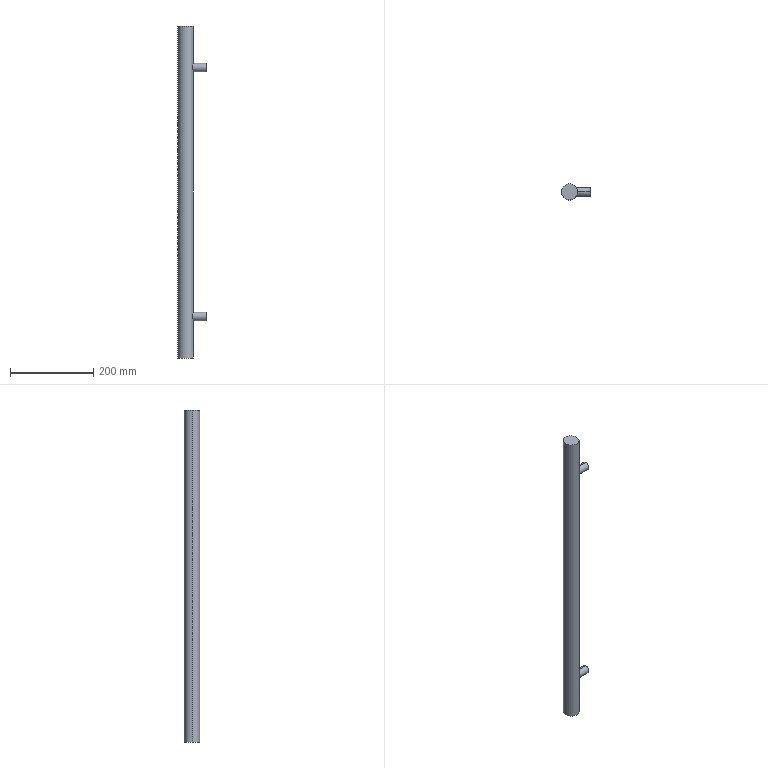Part | 1 solid | 16 faces | box 69 x 38 x 800 mm | volume 924183 mm3 | cylinder 10 | plane 6 | commonest cylinder face diameters 8 x4 20 x4 38 x2
STEP:
#1=CARTESIAN_POINT('',(20.,0.,-296.));
#2=VERTEX_POINT('',#1);
#3=CARTESIAN_POINT('',(20.,0.,-304.));
#4=VERTEX_POINT('',#3);
#5=CARTESIAN_POINT('',(20.,0.,-300.));
#6=DIRECTION('',(1.,0.,0.));
#7=DIRECTION('',(0.,0.,-1.));
#8=AXIS2_PLACEMENT_3D('',#5,#6,#7);
#9=CIRCLE('',#8,4.);
#10=EDGE_CURVE('',#2,#4,#9,.T.);
#11=ORIENTED_EDGE('',*,*,#10,.F.);
#12=CARTESIAN_POINT('',(50.,0.,-296.));
#13=VERTEX_POINT('',#12);
#14=CARTESIAN_POINT('',(20.,0.,-296.));
#15=DIRECTION('',(1.,0.,0.));
#16=VECTOR('',#15,1000.);
#17=LINE('',#14,#16);
#18=EDGE_CURVE('',#2,#13,#17,.T.);
#19=ORIENTED_EDGE('',*,*,#18,.T.);
#20=CARTESIAN_POINT('',(50.,0.,-304.));
#21=VERTEX_POINT('',#20);
#22=CARTESIAN_POINT('',(50.,0.,-300.));
#23=DIRECTION('',(1.,0.,0.));
#24=DIRECTION('',(0.,0.,-1.));
#25=AXIS2_PLACEMENT_3D('',#22,#23,#24);
#26=CIRCLE('',#25,4.);
#27=EDGE_CURVE('',#13,#21,#26,.T.);
#28=ORIENTED_EDGE('',*,*,#27,.T.);
#29=CARTESIAN_POINT('',(20.,0.,-304.));
#30=DIRECTION('',(1.,0.,0.));
#31=VECTOR('',#30,1000.);
#32=LINE('',#29,#31);
#33=EDGE_CURVE('',#4,#21,#32,.T.);
#34=ORIENTED_EDGE('',*,*,#33,.F.);
#35=EDGE_LOOP('',(#11,#19,#28,#34));
#36=FACE_OUTER_BOUND('',#35,.T.);
#37=CARTESIAN_POINT('',(20.,0.,-300.));
#38=DIRECTION('',(1.,0.,0.));
#39=DIRECTION('',(0.,0.,-1.));
#40=AXIS2_PLACEMENT_3D('',#37,#38,#39);
#41=CYLINDRICAL_SURFACE('',#40,4.);
#42=ADVANCED_FACE('',(#36),#41,.F.);
#43=CARTESIAN_POINT('',(20.,0.,304.));
#44=VERTEX_POINT('',#43);
#45=CARTESIAN_POINT('',(20.,0.,296.));
#46=VERTEX_POINT('',#45);
#47=CARTESIAN_POINT('',(20.,0.,300.));
#48=DIRECTION('',(1.,0.,0.));
#49=DIRECTION('',(0.,0.,-1.));
#50=AXIS2_PLACEMENT_3D('',#47,#48,#49);
#51=CIRCLE('',#50,4.);
#52=EDGE_CURVE('',#44,#46,#51,.T.);
#53=ORIENTED_EDGE('',*,*,#52,.F.);
#54=CARTESIAN_POINT('',(50.,0.,304.));
#55=VERTEX_POINT('',#54);
#56=CARTESIAN_POINT('',(20.,0.,304.));
#57=DIRECTION('',(1.,0.,0.));
#58=VECTOR('',#57,1000.);
#59=LINE('',#56,#58);
#60=EDGE_CURVE('',#44,#55,#59,.T.);
#61=ORIENTED_EDGE('',*,*,#60,.T.);
#62=CARTESIAN_POINT('',(50.,0.,296.));
#63=VERTEX_POINT('',#62);
#64=CARTESIAN_POINT('',(50.,0.,300.));
#65=DIRECTION('',(1.,0.,0.));
#66=DIRECTION('',(0.,0.,-1.));
#67=AXIS2_PLACEMENT_3D('',#64,#65,#66);
#68=CIRCLE('',#67,4.);
#69=EDGE_CURVE('',#55,#63,#68,.T.);
#70=ORIENTED_EDGE('',*,*,#69,.T.);
#71=CARTESIAN_POINT('',(20.,0.,296.));
#72=DIRECTION('',(1.,0.,0.));
#73=VECTOR('',#72,1000.);
#74=LINE('',#71,#73);
#75=EDGE_CURVE('',#46,#63,#74,.T.);
#76=ORIENTED_EDGE('',*,*,#75,.F.);
#77=EDGE_LOOP('',(#53,#61,#70,#76));
#78=FACE_OUTER_BOUND('',#77,.T.);
#79=CARTESIAN_POINT('',(20.,0.,300.));
#80=DIRECTION('',(1.,0.,0.));
#81=DIRECTION('',(0.,0.,-1.));
#82=AXIS2_PLACEMENT_3D('',#79,#80,#81);
#83=CYLINDRICAL_SURFACE('',#82,4.);
#84=ADVANCED_FACE('',(#78),#83,.F.);
#85=CARTESIAN_POINT('',(50.,0.,290.));
#86=VERTEX_POINT('',#85);
#87=CARTESIAN_POINT('',(50.,0.,310.));
#88=VERTEX_POINT('',#87);
#89=CARTESIAN_POINT('',(50.,0.,300.));
#90=DIRECTION('',(1.,0.,0.));
#91=DIRECTION('',(0.,0.,1.));
#92=AXIS2_PLACEMENT_3D('',#89,#90,#91);
#93=CIRCLE('',#92,10.);
#94=EDGE_CURVE('',#86,#88,#93,.T.);
#95=ORIENTED_EDGE('',*,*,#94,.F.);
#96=CARTESIAN_POINT('',(19.,0.,290.));
#97=VERTEX_POINT('',#96);
#98=CARTESIAN_POINT('',(50.,0.,290.));
#99=DIRECTION('',(-1.,0.,0.));
#100=VECTOR('',#99,1000.);
#101=LINE('',#98,#100);
#102=EDGE_CURVE('',#86,#97,#101,.T.);
#103=ORIENTED_EDGE('',*,*,#102,.T.);
#104=CARTESIAN_POINT('',(19.,0.,310.));
#105=VERTEX_POINT('',#104);
#106=CARTESIAN_POINT('',(19.,0.,290.));
#107=CARTESIAN_POINT('',(19.,0.3324,290.));
#108=CARTESIAN_POINT('',(18.991,0.6677,290.017));
#109=CARTESIAN_POINT('',(18.956,1.336,290.084));
#110=CARTESIAN_POINT('',(18.93,1.665,290.134));
#111=CARTESIAN_POINT('',(18.827,2.638,290.331));
#112=CARTESIAN_POINT('',(18.727,3.269,290.526));
#113=CARTESIAN_POINT('',(18.473,4.486,291.038));
#114=CARTESIAN_POINT('',(18.323,5.056,291.348));
#115=CARTESIAN_POINT('',(17.994,6.127,292.07));
#116=CARTESIAN_POINT('',(17.812,6.63,292.486));
#117=CARTESIAN_POINT('',(17.449,7.534,293.394));
#118=CARTESIAN_POINT('',(17.266,7.94,293.887));
#119=CARTESIAN_POINT('',(17.003,8.481,294.691));
#120=CARTESIAN_POINT('',(16.918,8.65,294.971));
#121=CARTESIAN_POINT('',(16.757,8.957,295.541));
#122=CARTESIAN_POINT('',(16.682,9.096,295.832));
#123=CARTESIAN_POINT('',(16.473,9.471,296.727));
#124=CARTESIAN_POINT('',(16.358,9.666,297.351));
#125=CARTESIAN_POINT('',(16.198,9.933,298.663));
#126=CARTESIAN_POINT('',(16.156,9.999,299.323));
#127=CARTESIAN_POINT('',(16.155,10.,300.317));
#128=CARTESIAN_POINT('',(16.165,9.984,300.65));
#129=CARTESIAN_POINT('',(16.206,9.919,301.315));
#130=CARTESIAN_POINT('',(16.236,9.869,301.649));
#131=CARTESIAN_POINT('',(16.354,9.672,302.624));
#132=CARTESIAN_POINT('',(16.469,9.479,303.251));
#133=CARTESIAN_POINT('',(16.68,9.099,304.161));
#134=CARTESIAN_POINT('',(16.757,8.958,304.457));
#135=CARTESIAN_POINT('',(16.917,8.65,305.027));
#136=CARTESIAN_POINT('',(17.002,8.484,305.303));
#137=CARTESIAN_POINT('',(17.176,8.126,305.838));
#138=CARTESIAN_POINT('',(17.266,7.934,306.096));
#139=CARTESIAN_POINT('',(17.448,7.524,306.595));
#140=CARTESIAN_POINT('',(17.541,7.306,306.835));
#141=CARTESIAN_POINT('',(17.814,6.626,307.517));
#142=CARTESIAN_POINT('',(17.992,6.133,307.925));
#143=CARTESIAN_POINT('',(18.239,5.33,308.468));
#144=CARTESIAN_POINT('',(18.319,5.05,308.638));
#145=CARTESIAN_POINT('',(18.468,4.474,308.949));
#146=CARTESIAN_POINT('',(18.537,4.18,309.09));
#147=CARTESIAN_POINT('',(18.725,3.279,309.47));
#148=CARTESIAN_POINT('',(18.825,2.654,309.664));
#149=CARTESIAN_POINT('',(18.929,1.675,309.864));
#150=CARTESIAN_POINT('',(18.956,1.341,309.915));
#151=CARTESIAN_POINT('',(18.991,0.673,309.983));
#152=CARTESIAN_POINT('',(19.,0.3365,310.));
#153=CARTESIAN_POINT('',(19.,0.,310.));
#154=B_SPLINE_CURVE_WITH_KNOTS('',3,(#106,#107,#108,#109,#110,#111,#112,#113,#114,#115,#116,#117,#118,#119,#120,#121,#122,#123,#124,#125,#126,#127,#128,#129,#130,#131,#132,#133,#134,#135,#136,#137,#138,#139,#140,#141,#142,#143,#144,#145,#146,#147,#148,#149,#150,#151,#152,#153),.UNSPECIFIED.,.F.,.F.,(4,2,2,2,2,2,2,2,2,2,2,2,2,2,2,2,2,2,2,2,2,2,2,4),(0.03188,0.03287,0.03386,0.03585,0.03784,0.03983,0.04182,0.04281,0.04381,0.04579,0.04778,0.04878,0.04977,0.05176,0.05275,0.05375,0.05474,0.05573,0.05772,0.05872,0.05971,0.0617,0.06269,0.06369),.UNSPECIFIED.);
#155=EDGE_CURVE('',#97,#105,#154,.T.);
#156=ORIENTED_EDGE('',*,*,#155,.T.);
#157=CARTESIAN_POINT('',(50.,0.,310.));
#158=DIRECTION('',(-1.,0.,0.));
#159=VECTOR('',#158,1000.);
#160=LINE('',#157,#159);
#161=EDGE_CURVE('',#88,#105,#160,.T.);
#162=ORIENTED_EDGE('',*,*,#161,.F.);
#163=EDGE_LOOP('',(#95,#103,#156,#162));
#164=FACE_OUTER_BOUND('',#163,.T.);
#165=CARTESIAN_POINT('',(50.,0.,300.));
#166=DIRECTION('',(-1.,0.,0.));
#167=DIRECTION('',(0.,0.,1.));
#168=AXIS2_PLACEMENT_3D('',#165,#166,#167);
#169=CYLINDRICAL_SURFACE('',#168,10.);
#170=ADVANCED_FACE('',(#164),#169,.T.);
#171=CARTESIAN_POINT('',(50.,0.,-310.));
#172=VERTEX_POINT('',#171);
#173=CARTESIAN_POINT('',(50.,0.,-290.));
#174=VERTEX_POINT('',#173);
#175=CARTESIAN_POINT('',(50.,0.,-300.));
#176=DIRECTION('',(1.,0.,0.));
#177=DIRECTION('',(0.,0.,-1.));
#178=AXIS2_PLACEMENT_3D('',#175,#176,#177);
#179=CIRCLE('',#178,10.);
#180=EDGE_CURVE('',#172,#174,#179,.T.);
#181=ORIENTED_EDGE('',*,*,#180,.F.);
#182=CARTESIAN_POINT('',(19.,0.,-310.));
#183=VERTEX_POINT('',#182);
#184=CARTESIAN_POINT('',(50.,0.,-310.));
#185=DIRECTION('',(-1.,0.,0.));
#186=VECTOR('',#185,1000.);
#187=LINE('',#184,#186);
#188=EDGE_CURVE('',#172,#183,#187,.T.);
#189=ORIENTED_EDGE('',*,*,#188,.T.);
#190=CARTESIAN_POINT('',(19.,0.,-290.));
#191=VERTEX_POINT('',#190);
#192=CARTESIAN_POINT('',(19.,0.,-310.));
#193=CARTESIAN_POINT('',(19.,0.3324,-310.));
#194=CARTESIAN_POINT('',(18.991,0.6677,-309.983));
#195=CARTESIAN_POINT('',(18.956,1.336,-309.916));
#196=CARTESIAN_POINT('',(18.93,1.665,-309.866));
#197=CARTESIAN_POINT('',(18.827,2.638,-309.669));
#198=CARTESIAN_POINT('',(18.727,3.269,-309.474));
#199=CARTESIAN_POINT('',(18.473,4.486,-308.962));
#200=CARTESIAN_POINT('',(18.323,5.056,-308.652));
#201=CARTESIAN_POINT('',(17.994,6.127,-307.93));
#202=CARTESIAN_POINT('',(17.812,6.63,-307.514));
#203=CARTESIAN_POINT('',(17.449,7.534,-306.606));
#204=CARTESIAN_POINT('',(17.266,7.94,-306.113));
#205=CARTESIAN_POINT('',(17.003,8.481,-305.309));
#206=CARTESIAN_POINT('',(16.918,8.65,-305.029));
#207=CARTESIAN_POINT('',(16.757,8.957,-304.459));
#208=CARTESIAN_POINT('',(16.682,9.096,-304.168));
#209=CARTESIAN_POINT('',(16.473,9.471,-303.273));
#210=CARTESIAN_POINT('',(16.358,9.666,-302.649));
#211=CARTESIAN_POINT('',(16.198,9.933,-301.337));
#212=CARTESIAN_POINT('',(16.156,9.999,-300.677));
#213=CARTESIAN_POINT('',(16.155,10.,-299.683));
#214=CARTESIAN_POINT('',(16.165,9.984,-299.35));
#215=CARTESIAN_POINT('',(16.206,9.919,-298.685));
#216=CARTESIAN_POINT('',(16.236,9.869,-298.351));
#217=CARTESIAN_POINT('',(16.354,9.672,-297.376));
#218=CARTESIAN_POINT('',(16.469,9.479,-296.749));
#219=CARTESIAN_POINT('',(16.68,9.099,-295.839));
#220=CARTESIAN_POINT('',(16.757,8.958,-295.543));
#221=CARTESIAN_POINT('',(16.917,8.65,-294.973));
#222=CARTESIAN_POINT('',(17.002,8.484,-294.697));
#223=CARTESIAN_POINT('',(17.176,8.126,-294.162));
#224=CARTESIAN_POINT('',(17.266,7.934,-293.904));
#225=CARTESIAN_POINT('',(17.448,7.524,-293.405));
#226=CARTESIAN_POINT('',(17.541,7.306,-293.165));
#227=CARTESIAN_POINT('',(17.814,6.626,-292.483));
#228=CARTESIAN_POINT('',(17.992,6.133,-292.075));
#229=CARTESIAN_POINT('',(18.239,5.33,-291.532));
#230=CARTESIAN_POINT('',(18.319,5.05,-291.362));
#231=CARTESIAN_POINT('',(18.468,4.474,-291.051));
#232=CARTESIAN_POINT('',(18.537,4.18,-290.91));
#233=CARTESIAN_POINT('',(18.725,3.279,-290.53));
#234=CARTESIAN_POINT('',(18.825,2.654,-290.336));
#235=CARTESIAN_POINT('',(18.929,1.675,-290.136));
#236=CARTESIAN_POINT('',(18.956,1.341,-290.085));
#237=CARTESIAN_POINT('',(18.991,0.673,-290.017));
#238=CARTESIAN_POINT('',(19.,0.3365,-290.));
#239=CARTESIAN_POINT('',(19.,0.,-290.));
#240=B_SPLINE_CURVE_WITH_KNOTS('',3,(#192,#193,#194,#195,#196,#197,#198,#199,#200,#201,#202,#203,#204,#205,#206,#207,#208,#209,#210,#211,#212,#213,#214,#215,#216,#217,#218,#219,#220,#221,#222,#223,#224,#225,#226,#227,#228,#229,#230,#231,#232,#233,#234,#235,#236,#237,#238,#239),.UNSPECIFIED.,.F.,.F.,(4,2,2,2,2,2,2,2,2,2,2,2,2,2,2,2,2,2,2,2,2,2,2,4),(0.03188,0.03287,0.03386,0.03585,0.03784,0.03983,0.04182,0.04281,0.04381,0.04579,0.04778,0.04878,0.04977,0.05176,0.05275,0.05375,0.05474,0.05573,0.05772,0.05872,0.05971,0.0617,0.06269,0.06369),.UNSPECIFIED.);
#241=EDGE_CURVE('',#183,#191,#240,.T.);
#242=ORIENTED_EDGE('',*,*,#241,.T.);
#243=CARTESIAN_POINT('',(50.,0.,-290.));
#244=DIRECTION('',(-1.,0.,0.));
#245=VECTOR('',#244,1000.);
#246=LINE('',#243,#245);
#247=EDGE_CURVE('',#174,#191,#246,.T.);
#248=ORIENTED_EDGE('',*,*,#247,.F.);
#249=EDGE_LOOP('',(#181,#189,#242,#248));
#250=FACE_OUTER_BOUND('',#249,.T.);
#251=CARTESIAN_POINT('',(50.,0.,-300.));
#252=DIRECTION('',(-1.,0.,0.));
#253=DIRECTION('',(0.,0.,1.));
#254=AXIS2_PLACEMENT_3D('',#251,#252,#253);
#255=CYLINDRICAL_SURFACE('',#254,10.);
#256=ADVANCED_FACE('',(#250),#255,.T.);
#257=CARTESIAN_POINT('',(19.,0.,400.));
#258=VERTEX_POINT('',#257);
#259=CARTESIAN_POINT('',(-19.,0.,400.));
#260=VERTEX_POINT('',#259);
#261=CARTESIAN_POINT('',(0.,0.,400.));
#262=DIRECTION('',(0.,0.,1.));
#263=DIRECTION('',(1.,0.,0.));
#264=AXIS2_PLACEMENT_3D('',#261,#262,#263);
#265=CIRCLE('',#264,19.);
#266=EDGE_CURVE('',#258,#260,#265,.T.);
#267=ORIENTED_EDGE('',*,*,#266,.F.);
#268=CARTESIAN_POINT('',(19.,0.,400.));
#269=DIRECTION('',(0.,0.,-1.));
#270=VECTOR('',#269,1000.);
#271=LINE('',#268,#270);
#272=EDGE_CURVE('',#258,#105,#271,.T.);
#273=ORIENTED_EDGE('',*,*,#272,.T.);
#274=ORIENTED_EDGE('',*,*,#155,.F.);
#275=CARTESIAN_POINT('',(19.,0.,400.));
#276=DIRECTION('',(0.,0.,-1.));
#277=VECTOR('',#276,1000.);
#278=LINE('',#275,#277);
#279=EDGE_CURVE('',#97,#191,#278,.T.);
#280=ORIENTED_EDGE('',*,*,#279,.T.);
#281=ORIENTED_EDGE('',*,*,#241,.F.);
#282=CARTESIAN_POINT('',(19.,0.,-400.));
#283=VERTEX_POINT('',#282);
#284=CARTESIAN_POINT('',(19.,0.,400.));
#285=DIRECTION('',(0.,0.,-1.));
#286=VECTOR('',#285,1000.);
#287=LINE('',#284,#286);
#288=EDGE_CURVE('',#183,#283,#287,.T.);
#289=ORIENTED_EDGE('',*,*,#288,.T.);
#290=CARTESIAN_POINT('',(-19.,0.,-400.));
#291=VERTEX_POINT('',#290);
#292=CARTESIAN_POINT('',(0.,0.,-400.));
#293=DIRECTION('',(0.,0.,1.));
#294=DIRECTION('',(1.,0.,0.));
#295=AXIS2_PLACEMENT_3D('',#292,#293,#294);
#296=CIRCLE('',#295,19.);
#297=EDGE_CURVE('',#283,#291,#296,.T.);
#298=ORIENTED_EDGE('',*,*,#297,.T.);
#299=CARTESIAN_POINT('',(-19.,0.,400.));
#300=DIRECTION('',(0.,0.,-1.));
#301=VECTOR('',#300,1000.);
#302=LINE('',#299,#301);
#303=EDGE_CURVE('',#260,#291,#302,.T.);
#304=ORIENTED_EDGE('',*,*,#303,.F.);
#305=EDGE_LOOP('',(#267,#273,#274,#280,#281,#289,#298,#304));
#306=FACE_OUTER_BOUND('',#305,.T.);
#307=CARTESIAN_POINT('',(0.,0.,400.));
#308=DIRECTION('',(0.,0.,-1.));
#309=DIRECTION('',(-1.,0.,0.));
#310=AXIS2_PLACEMENT_3D('',#307,#308,#309);
#311=CYLINDRICAL_SURFACE('',#310,19.);
#312=ADVANCED_FACE('',(#306),#311,.T.);
#313=ORIENTED_EDGE('',*,*,#272,.F.);
#314=CARTESIAN_POINT('',(0.,0.,400.));
#315=DIRECTION('',(0.,0.,1.));
#316=DIRECTION('',(1.,0.,0.));
#317=AXIS2_PLACEMENT_3D('',#314,#315,#316);
#318=CIRCLE('',#317,19.);
#319=EDGE_CURVE('',#260,#258,#318,.T.);
#320=ORIENTED_EDGE('',*,*,#319,.F.);
#321=ORIENTED_EDGE('',*,*,#303,.T.);
#322=CARTESIAN_POINT('',(0.,0.,-400.));
#323=DIRECTION('',(0.,0.,1.));
#324=DIRECTION('',(1.,0.,0.));
#325=AXIS2_PLACEMENT_3D('',#322,#323,#324);
#326=CIRCLE('',#325,19.);
#327=EDGE_CURVE('',#291,#283,#326,.T.);
#328=ORIENTED_EDGE('',*,*,#327,.T.);
#329=ORIENTED_EDGE('',*,*,#288,.F.);
#330=CARTESIAN_POINT('',(19.,0.,-290.));
#331=CARTESIAN_POINT('',(19.,-0.6745,-290.));
#332=CARTESIAN_POINT('',(18.964,-1.335,-290.068));
#333=CARTESIAN_POINT('',(18.862,-2.308,-290.264));
#334=CARTESIAN_POINT('',(18.82,-2.629,-290.346));
#335=CARTESIAN_POINT('',(18.72,-3.264,-290.542));
#336=CARTESIAN_POINT('',(18.663,-3.576,-290.655));
#337=CARTESIAN_POINT('',(18.474,-4.481,-291.036));
#338=CARTESIAN_POINT('',(18.325,-5.052,-291.345));
#339=CARTESIAN_POINT('',(18.076,-5.86,-291.891));
#340=CARTESIAN_POINT('',(17.989,-6.121,-292.086));
#341=CARTESIAN_POINT('',(17.812,-6.618,-292.496));
#342=CARTESIAN_POINT('',(17.722,-6.854,-292.712));
#343=CARTESIAN_POINT('',(17.541,-7.306,-293.165));
#344=CARTESIAN_POINT('',(17.449,-7.522,-293.402));
#345=CARTESIAN_POINT('',(17.267,-7.93,-293.899));
#346=CARTESIAN_POINT('',(17.177,-8.124,-294.16));
#347=CARTESIAN_POINT('',(16.914,-8.664,-294.965));
#348=CARTESIAN_POINT('',(16.752,-8.969,-295.531));
#349=CARTESIAN_POINT('',(16.543,-9.346,-296.429));
#350=CARTESIAN_POINT('',(16.479,-9.458,-296.736));
#351=CARTESIAN_POINT('',(16.365,-9.653,-297.369));
#352=CARTESIAN_POINT('',(16.316,-9.736,-297.693));
#353=CARTESIAN_POINT('',(16.198,-9.932,-298.664));
#354=CARTESIAN_POINT('',(16.156,-9.999,-299.322));
#355=CARTESIAN_POINT('',(16.155,-10.,-300.322));
#356=CARTESIAN_POINT('',(16.166,-9.984,-300.661));
#357=CARTESIAN_POINT('',(16.206,-9.917,-301.327));
#358=CARTESIAN_POINT('',(16.237,-9.868,-301.655));
#359=CARTESIAN_POINT('',(16.316,-9.737,-302.303));
#360=CARTESIAN_POINT('',(16.364,-9.656,-302.623));
#361=CARTESIAN_POINT('',(16.477,-9.462,-303.254));
#362=CARTESIAN_POINT('',(16.542,-9.348,-303.566));
#363=CARTESIAN_POINT('',(16.753,-8.968,-304.472));
#364=CARTESIAN_POINT('',(16.916,-8.661,-305.041));
#365=CARTESIAN_POINT('',(17.179,-8.12,-305.846));
#366=CARTESIAN_POINT('',(17.27,-7.925,-306.107));
#367=CARTESIAN_POINT('',(17.452,-7.515,-306.605));
#368=CARTESIAN_POINT('',(17.543,-7.3,-306.842));
#369=CARTESIAN_POINT('',(17.816,-6.621,-307.522));
#370=CARTESIAN_POINT('',(17.995,-6.125,-307.932));
#371=CARTESIAN_POINT('',(18.328,-5.042,-308.66));
#372=CARTESIAN_POINT('',(18.476,-4.472,-308.968));
#373=CARTESIAN_POINT('',(18.664,-3.571,-309.346));
#374=CARTESIAN_POINT('',(18.72,-3.263,-309.458));
#375=CARTESIAN_POINT('',(18.82,-2.632,-309.653));
#376=CARTESIAN_POINT('',(18.862,-2.306,-309.736));
#377=CARTESIAN_POINT('',(18.965,-1.326,-309.934));
#378=CARTESIAN_POINT('',(19.,-0.6662,-310.));
#379=CARTESIAN_POINT('',(19.,0.,-310.));
#380=B_SPLINE_CURVE_WITH_KNOTS('',3,(#330,#331,#332,#333,#334,#335,#336,#337,#338,#339,#340,#341,#342,#343,#344,#345,#346,#347,#348,#349,#350,#351,#352,#353,#354,#355,#356,#357,#358,#359,#360,#361,#362,#363,#364,#365,#366,#367,#368,#369,#370,#371,#372,#373,#374,#375,#376,#377,#378,#379),.UNSPECIFIED.,.F.,.F.,(4,2,2,2,2,2,2,2,2,2,2,2,2,2,2,2,2,2,2,2,2,2,2,2,4),(0.,0.001992,0.002988,0.003985,0.005977,0.006973,0.007969,0.008965,0.009961,0.01195,0.01295,0.01395,0.01594,0.01693,0.01793,0.01893,0.01992,0.02192,0.02291,0.02391,0.0259,0.02789,0.02889,0.02988,0.03188),.UNSPECIFIED.);
#381=EDGE_CURVE('',#191,#183,#380,.T.);
#382=ORIENTED_EDGE('',*,*,#381,.F.);
#383=ORIENTED_EDGE('',*,*,#279,.F.);
#384=CARTESIAN_POINT('',(19.,0.,310.));
#385=CARTESIAN_POINT('',(19.,-0.6745,310.));
#386=CARTESIAN_POINT('',(18.964,-1.335,309.932));
#387=CARTESIAN_POINT('',(18.862,-2.308,309.736));
#388=CARTESIAN_POINT('',(18.82,-2.629,309.654));
#389=CARTESIAN_POINT('',(18.72,-3.264,309.458));
#390=CARTESIAN_POINT('',(18.663,-3.576,309.345));
#391=CARTESIAN_POINT('',(18.474,-4.481,308.964));
#392=CARTESIAN_POINT('',(18.325,-5.052,308.655));
#393=CARTESIAN_POINT('',(18.076,-5.86,308.109));
#394=CARTESIAN_POINT('',(17.989,-6.121,307.914));
#395=CARTESIAN_POINT('',(17.812,-6.618,307.504));
#396=CARTESIAN_POINT('',(17.722,-6.854,307.288));
#397=CARTESIAN_POINT('',(17.541,-7.306,306.835));
#398=CARTESIAN_POINT('',(17.449,-7.522,306.598));
#399=CARTESIAN_POINT('',(17.267,-7.93,306.101));
#400=CARTESIAN_POINT('',(17.177,-8.124,305.84));
#401=CARTESIAN_POINT('',(16.914,-8.664,305.035));
#402=CARTESIAN_POINT('',(16.752,-8.969,304.469));
#403=CARTESIAN_POINT('',(16.543,-9.346,303.571));
#404=CARTESIAN_POINT('',(16.479,-9.458,303.264));
#405=CARTESIAN_POINT('',(16.365,-9.653,302.631));
#406=CARTESIAN_POINT('',(16.316,-9.736,302.307));
#407=CARTESIAN_POINT('',(16.198,-9.932,301.336));
#408=CARTESIAN_POINT('',(16.156,-9.999,300.678));
#409=CARTESIAN_POINT('',(16.155,-10.,299.678));
#410=CARTESIAN_POINT('',(16.166,-9.984,299.339));
#411=CARTESIAN_POINT('',(16.206,-9.917,298.673));
#412=CARTESIAN_POINT('',(16.237,-9.868,298.345));
#413=CARTESIAN_POINT('',(16.316,-9.737,297.697));
#414=CARTESIAN_POINT('',(16.364,-9.656,297.377));
#415=CARTESIAN_POINT('',(16.477,-9.462,296.746));
#416=CARTESIAN_POINT('',(16.542,-9.348,296.434));
#417=CARTESIAN_POINT('',(16.753,-8.968,295.528));
#418=CARTESIAN_POINT('',(16.916,-8.661,294.959));
#419=CARTESIAN_POINT('',(17.179,-8.12,294.154));
#420=CARTESIAN_POINT('',(17.27,-7.925,293.893));
#421=CARTESIAN_POINT('',(17.452,-7.515,293.395));
#422=CARTESIAN_POINT('',(17.543,-7.3,293.158));
#423=CARTESIAN_POINT('',(17.816,-6.621,292.478));
#424=CARTESIAN_POINT('',(17.995,-6.125,292.068));
#425=CARTESIAN_POINT('',(18.328,-5.042,291.34));
#426=CARTESIAN_POINT('',(18.476,-4.472,291.032));
#427=CARTESIAN_POINT('',(18.664,-3.571,290.654));
#428=CARTESIAN_POINT('',(18.72,-3.263,290.542));
#429=CARTESIAN_POINT('',(18.82,-2.632,290.347));
#430=CARTESIAN_POINT('',(18.862,-2.306,290.264));
#431=CARTESIAN_POINT('',(18.965,-1.326,290.066));
#432=CARTESIAN_POINT('',(19.,-0.6662,290.));
#433=CARTESIAN_POINT('',(19.,0.,290.));
#434=B_SPLINE_CURVE_WITH_KNOTS('',3,(#384,#385,#386,#387,#388,#389,#390,#391,#392,#393,#394,#395,#396,#397,#398,#399,#400,#401,#402,#403,#404,#405,#406,#407,#408,#409,#410,#411,#412,#413,#414,#415,#416,#417,#418,#419,#420,#421,#422,#423,#424,#425,#426,#427,#428,#429,#430,#431,#432,#433),.UNSPECIFIED.,.F.,.F.,(4,2,2,2,2,2,2,2,2,2,2,2,2,2,2,2,2,2,2,2,2,2,2,2,4),(0.,0.001992,0.002988,0.003985,0.005977,0.006973,0.007969,0.008965,0.009961,0.01195,0.01295,0.01395,0.01594,0.01693,0.01793,0.01893,0.01992,0.02192,0.02291,0.02391,0.0259,0.02789,0.02889,0.02988,0.03188),.UNSPECIFIED.);
#435=EDGE_CURVE('',#105,#97,#434,.T.);
#436=ORIENTED_EDGE('',*,*,#435,.F.);
#437=EDGE_LOOP('',(#313,#320,#321,#328,#329,#382,#383,#436));
#438=FACE_OUTER_BOUND('',#437,.T.);
#439=CARTESIAN_POINT('',(0.,0.,400.));
#440=DIRECTION('',(0.,0.,-1.));
#441=DIRECTION('',(-1.,0.,0.));
#442=AXIS2_PLACEMENT_3D('',#439,#440,#441);
#443=CYLINDRICAL_SURFACE('',#442,19.);
#444=ADVANCED_FACE('',(#438),#443,.T.);
#445=ORIENTED_EDGE('',*,*,#319,.T.);
#446=ORIENTED_EDGE('',*,*,#266,.T.);
#447=EDGE_LOOP('',(#445,#446));
#448=FACE_OUTER_BOUND('',#447,.T.);
#449=CARTESIAN_POINT('',(0.,0.,400.));
#450=DIRECTION('',(0.,0.,1.));
#451=DIRECTION('',(1.,0.,0.));
#452=AXIS2_PLACEMENT_3D('',#449,#450,#451);
#453=PLANE('',#452);
#454=ADVANCED_FACE('',(#448),#453,.T.);
#455=ORIENTED_EDGE('',*,*,#327,.F.);
#456=ORIENTED_EDGE('',*,*,#297,.F.);
#457=EDGE_LOOP('',(#455,#456));
#458=FACE_OUTER_BOUND('',#457,.T.);
#459=CARTESIAN_POINT('',(0.,0.,-400.));
#460=DIRECTION('',(0.,0.,1.));
#461=DIRECTION('',(1.,0.,0.));
#462=AXIS2_PLACEMENT_3D('',#459,#460,#461);
#463=PLANE('',#462);
#464=ADVANCED_FACE('',(#458),#463,.F.);
#465=ORIENTED_EDGE('',*,*,#188,.F.);
#466=CARTESIAN_POINT('',(50.,0.,-300.));
#467=DIRECTION('',(1.,0.,0.));
#468=DIRECTION('',(0.,0.,-1.));
#469=AXIS2_PLACEMENT_3D('',#466,#467,#468);
#470=CIRCLE('',#469,10.);
#471=EDGE_CURVE('',#174,#172,#470,.T.);
#472=ORIENTED_EDGE('',*,*,#471,.F.);
#473=ORIENTED_EDGE('',*,*,#247,.T.);
#474=ORIENTED_EDGE('',*,*,#381,.T.);
#475=EDGE_LOOP('',(#465,#472,#473,#474));
#476=FACE_OUTER_BOUND('',#475,.T.);
#477=CARTESIAN_POINT('',(50.,0.,-300.));
#478=DIRECTION('',(-1.,0.,0.));
#479=DIRECTION('',(0.,0.,1.));
#480=AXIS2_PLACEMENT_3D('',#477,#478,#479);
#481=CYLINDRICAL_SURFACE('',#480,10.);
#482=ADVANCED_FACE('',(#476),#481,.T.);
#483=CARTESIAN_POINT('',(50.,0.,-300.));
#484=DIRECTION('',(1.,0.,0.));
#485=DIRECTION('',(0.,0.,-1.));
#486=AXIS2_PLACEMENT_3D('',#483,#484,#485);
#487=CIRCLE('',#486,4.);
#488=EDGE_CURVE('',#21,#13,#487,.T.);
#489=ORIENTED_EDGE('',*,*,#488,.F.);
#490=ORIENTED_EDGE('',*,*,#27,.F.);
#491=EDGE_LOOP('',(#489,#490));
#492=FACE_BOUND('',#491,.T.);
#493=ORIENTED_EDGE('',*,*,#471,.T.);
#494=ORIENTED_EDGE('',*,*,#180,.T.);
#495=EDGE_LOOP('',(#493,#494));
#496=FACE_OUTER_BOUND('',#495,.T.);
#497=CARTESIAN_POINT('',(50.,0.,-300.));
#498=DIRECTION('',(1.,0.,0.));
#499=DIRECTION('',(0.,0.,-1.));
#500=AXIS2_PLACEMENT_3D('',#497,#498,#499);
#501=PLANE('',#500);
#502=ADVANCED_FACE('',(#492,#496),#501,.T.);
#503=ORIENTED_EDGE('',*,*,#102,.F.);
#504=CARTESIAN_POINT('',(50.,0.,300.));
#505=DIRECTION('',(1.,0.,0.));
#506=DIRECTION('',(0.,0.,1.));
#507=AXIS2_PLACEMENT_3D('',#504,#505,#506);
#508=CIRCLE('',#507,10.);
#509=EDGE_CURVE('',#88,#86,#508,.T.);
#510=ORIENTED_EDGE('',*,*,#509,.F.);
#511=ORIENTED_EDGE('',*,*,#161,.T.);
#512=ORIENTED_EDGE('',*,*,#435,.T.);
#513=EDGE_LOOP('',(#503,#510,#511,#512));
#514=FACE_OUTER_BOUND('',#513,.T.);
#515=CARTESIAN_POINT('',(50.,0.,300.));
#516=DIRECTION('',(-1.,0.,0.));
#517=DIRECTION('',(0.,0.,1.));
#518=AXIS2_PLACEMENT_3D('',#515,#516,#517);
#519=CYLINDRICAL_SURFACE('',#518,10.);
#520=ADVANCED_FACE('',(#514),#519,.T.);
#521=CARTESIAN_POINT('',(50.,0.,300.));
#522=DIRECTION('',(1.,0.,0.));
#523=DIRECTION('',(0.,0.,-1.));
#524=AXIS2_PLACEMENT_3D('',#521,#522,#523);
#525=CIRCLE('',#524,4.);
#526=EDGE_CURVE('',#63,#55,#525,.T.);
#527=ORIENTED_EDGE('',*,*,#526,.F.);
#528=ORIENTED_EDGE('',*,*,#69,.F.);
#529=EDGE_LOOP('',(#527,#528));
#530=FACE_BOUND('',#529,.T.);
#531=ORIENTED_EDGE('',*,*,#509,.T.);
#532=ORIENTED_EDGE('',*,*,#94,.T.);
#533=EDGE_LOOP('',(#531,#532));
#534=FACE_OUTER_BOUND('',#533,.T.);
#535=CARTESIAN_POINT('',(50.,0.,300.));
#536=DIRECTION('',(-1.,0.,0.));
#537=DIRECTION('',(0.,0.,1.));
#538=AXIS2_PLACEMENT_3D('',#535,#536,#537);
#539=PLANE('',#538);
#540=ADVANCED_FACE('',(#530,#534),#539,.F.);
#541=ORIENTED_EDGE('',*,*,#60,.F.);
#542=CARTESIAN_POINT('',(20.,0.,300.));
#543=DIRECTION('',(1.,0.,0.));
#544=DIRECTION('',(0.,0.,-1.));
#545=AXIS2_PLACEMENT_3D('',#542,#543,#544);
#546=CIRCLE('',#545,4.);
#547=EDGE_CURVE('',#46,#44,#546,.T.);
#548=ORIENTED_EDGE('',*,*,#547,.F.);
#549=ORIENTED_EDGE('',*,*,#75,.T.);
#550=ORIENTED_EDGE('',*,*,#526,.T.);
#551=EDGE_LOOP('',(#541,#548,#549,#550));
#552=FACE_OUTER_BOUND('',#551,.T.);
#553=CARTESIAN_POINT('',(20.,0.,300.));
#554=DIRECTION('',(1.,0.,0.));
#555=DIRECTION('',(0.,0.,-1.));
#556=AXIS2_PLACEMENT_3D('',#553,#554,#555);
#557=CYLINDRICAL_SURFACE('',#556,4.);
#558=ADVANCED_FACE('',(#552),#557,.F.);
#559=ORIENTED_EDGE('',*,*,#547,.T.);
#560=ORIENTED_EDGE('',*,*,#52,.T.);
#561=EDGE_LOOP('',(#559,#560));
#562=FACE_OUTER_BOUND('',#561,.T.);
#563=CARTESIAN_POINT('',(20.,0.,300.));
#564=DIRECTION('',(1.,0.,0.));
#565=DIRECTION('',(0.,0.,-1.));
#566=AXIS2_PLACEMENT_3D('',#563,#564,#565);
#567=PLANE('',#566);
#568=ADVANCED_FACE('',(#562),#567,.T.);
#569=ORIENTED_EDGE('',*,*,#18,.F.);
#570=CARTESIAN_POINT('',(20.,0.,-300.));
#571=DIRECTION('',(1.,0.,0.));
#572=DIRECTION('',(0.,0.,-1.));
#573=AXIS2_PLACEMENT_3D('',#570,#571,#572);
#574=CIRCLE('',#573,4.);
#575=EDGE_CURVE('',#4,#2,#574,.T.);
#576=ORIENTED_EDGE('',*,*,#575,.F.);
#577=ORIENTED_EDGE('',*,*,#33,.T.);
#578=ORIENTED_EDGE('',*,*,#488,.T.);
#579=EDGE_LOOP('',(#569,#576,#577,#578));
#580=FACE_OUTER_BOUND('',#579,.T.);
#581=CARTESIAN_POINT('',(20.,0.,-300.));
#582=DIRECTION('',(1.,0.,0.));
#583=DIRECTION('',(0.,0.,-1.));
#584=AXIS2_PLACEMENT_3D('',#581,#582,#583);
#585=CYLINDRICAL_SURFACE('',#584,4.);
#586=ADVANCED_FACE('',(#580),#585,.F.);
#587=ORIENTED_EDGE('',*,*,#575,.T.);
#588=ORIENTED_EDGE('',*,*,#10,.T.);
#589=EDGE_LOOP('',(#587,#588));
#590=FACE_OUTER_BOUND('',#589,.T.);
#591=CARTESIAN_POINT('',(20.,0.,-300.));
#592=DIRECTION('',(1.,0.,0.));
#593=DIRECTION('',(0.,0.,-1.));
#594=AXIS2_PLACEMENT_3D('',#591,#592,#593);
#595=PLANE('',#594);
#596=ADVANCED_FACE('',(#590),#595,.T.);
#597=CLOSED_SHELL('',(#42,#84,#170,#256,#312,#444,#454,#464,#482,#502,#520,#540,#558,#568,#586,#596));
#598=MANIFOLD_SOLID_BREP('',#597);
#599=CARTESIAN_POINT('',(0.,0.,0.));
#600=DIRECTION('',(0.,0.,1.));
#601=DIRECTION('',(1.,0.,0.));
#602=AXIS2_PLACEMENT_3D('',#599,#600,#601);
#603=(LENGTH_UNIT()NAMED_UNIT(*)SI_UNIT(.MILLI.,.METRE.));
#604=UNCERTAINTY_MEASURE_WITH_UNIT(LENGTH_MEASURE(0.00001),#603,'','');
#605=(NAMED_UNIT(*)PLANE_ANGLE_UNIT()SI_UNIT($,.RADIAN.));
#606=(NAMED_UNIT(*)SI_UNIT($,.STERADIAN.)SOLID_ANGLE_UNIT());
#607=(GEOMETRIC_REPRESENTATION_CONTEXT(3)GLOBAL_UNCERTAINTY_ASSIGNED_CONTEXT((#604))GLOBAL_UNIT_ASSIGNED_CONTEXT((#603,#605,#606))REPRESENTATION_CONTEXT('',''));
#608=ADVANCED_BREP_SHAPE_REPRESENTATION('',(#598,#602),#607);